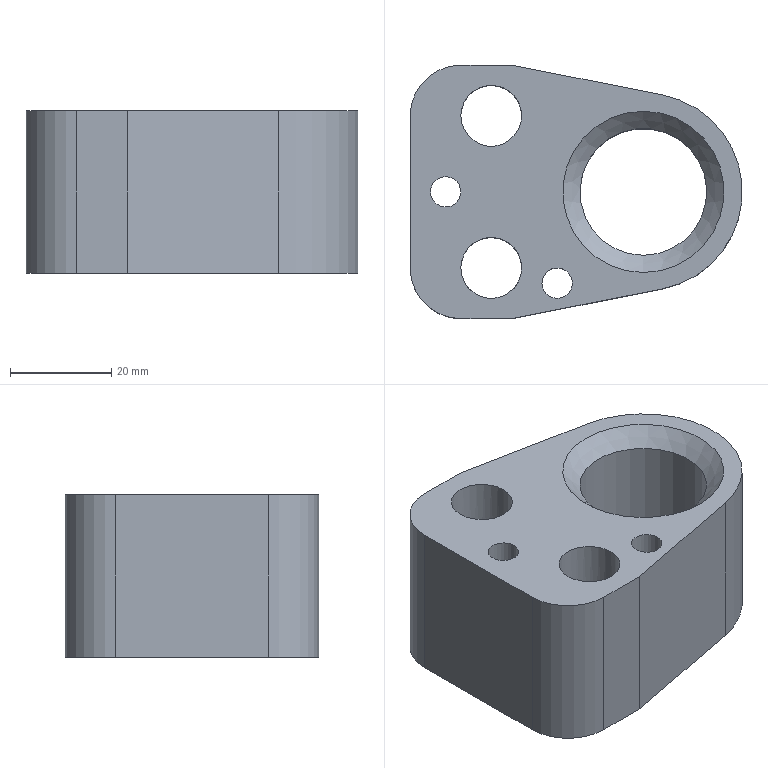Part | NX | features solid 2 | 1 solid | 24 faces | box 65.5 x 50 x 32 mm | volume 58243 mm3 | cylinder 12 | plane 11 | cone 1 | commonest cylinder face diameters 6 x2 8 x2 12 x2 17 x2 20 x2 25 x1
STEP:
#1=CARTESIAN_POINT('',(-607.367,572.653,75.));
#2=VERTEX_POINT('',#1);
#3=CARTESIAN_POINT('',(-607.367,576.653,75.));
#4=DIRECTION('',(0.,0.,-1.));
#5=DIRECTION('',(0.,-1.,0.));
#6=AXIS2_PLACEMENT_3D('',#3,#4,#5);
#7=CIRCLE('',#6,4.);
#8=EDGE_CURVE('',#2,#2,#7,.F.);
#9=ORIENTED_EDGE('',*,*,#8,.T.);
#10=EDGE_LOOP('',(#9));
#11=FACE_BOUND('',#10,.T.);
#12=CARTESIAN_POINT('',(-606.867,591.653,75.));
#13=VERTEX_POINT('',#12);
#14=CARTESIAN_POINT('',(-598.367,591.653,75.));
#15=DIRECTION('',(0.,0.,1.));
#16=DIRECTION('',(-1.,0.,0.));
#17=AXIS2_PLACEMENT_3D('',#14,#15,#16);
#18=CIRCLE('',#17,8.5);
#19=EDGE_CURVE('',#13,#13,#18,.T.);
#20=ORIENTED_EDGE('',*,*,#19,.T.);
#21=EDGE_LOOP('',(#20));
#22=FACE_BOUND('',#21,.T.);
#23=CARTESIAN_POINT('',(-606.867,561.653,75.));
#24=VERTEX_POINT('',#23);
#25=CARTESIAN_POINT('',(-598.367,561.653,75.));
#26=DIRECTION('',(0.,0.,1.));
#27=DIRECTION('',(-1.,0.,0.));
#28=AXIS2_PLACEMENT_3D('',#25,#26,#27);
#29=CIRCLE('',#28,8.5);
#30=EDGE_CURVE('',#24,#24,#29,.T.);
#31=ORIENTED_EDGE('',*,*,#30,.T.);
#32=EDGE_LOOP('',(#31));
#33=FACE_BOUND('',#32,.T.);
#34=CARTESIAN_POINT('',(-568.367,564.153,75.));
#35=VERTEX_POINT('',#34);
#36=CARTESIAN_POINT('',(-568.367,576.653,75.));
#37=DIRECTION('',(0.,0.,-1.));
#38=DIRECTION('',(0.,-1.,0.));
#39=AXIS2_PLACEMENT_3D('',#36,#37,#38);
#40=CIRCLE('',#39,12.5);
#41=EDGE_CURVE('',#35,#35,#40,.T.);
#42=ORIENTED_EDGE('',*,*,#41,.F.);
#43=EDGE_LOOP('',(#42));
#44=FACE_BOUND('',#43,.T.);
#45=CARTESIAN_POINT('',(-604.367,601.653,75.));
#46=VERTEX_POINT('',#45);
#47=CARTESIAN_POINT('',(-614.367,591.653,75.));
#48=VERTEX_POINT('',#47);
#49=CARTESIAN_POINT('',(-604.367,591.653,75.));
#50=DIRECTION('',(0.,0.,1.));
#51=DIRECTION('',(-1.,0.,0.));
#52=AXIS2_PLACEMENT_3D('',#49,#50,#51);
#53=CIRCLE('',#52,10.);
#54=EDGE_CURVE('',#46,#48,#53,.T.);
#55=ORIENTED_EDGE('',*,*,#54,.F.);
#56=CARTESIAN_POINT('',(-594.367,601.653,75.));
#57=VERTEX_POINT('',#56);
#58=CARTESIAN_POINT('',(-594.367,601.653,75.));
#59=DIRECTION('',(-1.,0.,0.));
#60=VECTOR('',#59,1000.);
#61=LINE('',#58,#60);
#62=EDGE_CURVE('',#57,#46,#61,.T.);
#63=ORIENTED_EDGE('',*,*,#62,.F.);
#64=CARTESIAN_POINT('',(-564.595,595.785,75.));
#65=VERTEX_POINT('',#64);
#66=CARTESIAN_POINT('',(-564.595,595.785,75.));
#67=DIRECTION('',(-0.9811,0.1934,0.));
#68=VECTOR('',#67,1000.);
#69=LINE('',#66,#68);
#70=EDGE_CURVE('',#65,#57,#69,.T.);
#71=ORIENTED_EDGE('',*,*,#70,.F.);
#72=CARTESIAN_POINT('',(-564.595,557.521,75.));
#73=VERTEX_POINT('',#72);
#74=CARTESIAN_POINT('',(-568.367,576.653,75.));
#75=DIRECTION('',(0.,0.,1.));
#76=DIRECTION('',(-1.,0.,0.));
#77=AXIS2_PLACEMENT_3D('',#74,#75,#76);
#78=CIRCLE('',#77,19.5);
#79=EDGE_CURVE('',#73,#65,#78,.T.);
#80=ORIENTED_EDGE('',*,*,#79,.F.);
#81=CARTESIAN_POINT('',(-594.367,551.653,75.));
#82=VERTEX_POINT('',#81);
#83=CARTESIAN_POINT('',(-564.595,557.521,75.));
#84=DIRECTION('',(-0.9811,-0.1934,0.));
#85=VECTOR('',#84,1000.);
#86=LINE('',#83,#85);
#87=EDGE_CURVE('',#73,#82,#86,.T.);
#88=ORIENTED_EDGE('',*,*,#87,.T.);
#89=CARTESIAN_POINT('',(-604.367,551.653,75.));
#90=VERTEX_POINT('',#89);
#91=CARTESIAN_POINT('',(-594.367,551.653,75.));
#92=DIRECTION('',(-1.,0.,0.));
#93=VECTOR('',#92,1000.);
#94=LINE('',#91,#93);
#95=EDGE_CURVE('',#82,#90,#94,.T.);
#96=ORIENTED_EDGE('',*,*,#95,.T.);
#97=CARTESIAN_POINT('',(-614.367,561.653,75.));
#98=VERTEX_POINT('',#97);
#99=CARTESIAN_POINT('',(-604.367,561.653,75.));
#100=DIRECTION('',(0.,0.,1.));
#101=DIRECTION('',(-1.,0.,0.));
#102=AXIS2_PLACEMENT_3D('',#99,#100,#101);
#103=CIRCLE('',#102,10.);
#104=EDGE_CURVE('',#98,#90,#103,.T.);
#105=ORIENTED_EDGE('',*,*,#104,.F.);
#106=CARTESIAN_POINT('',(-614.367,561.653,75.));
#107=DIRECTION('',(0.,1.,0.));
#108=VECTOR('',#107,1000.);
#109=LINE('',#106,#108);
#110=EDGE_CURVE('',#98,#48,#109,.T.);
#111=ORIENTED_EDGE('',*,*,#110,.T.);
#112=EDGE_LOOP('',(#55,#63,#71,#80,#88,#96,#105,#111));
#113=FACE_BOUND('',#112,.T.);
#114=CARTESIAN_POINT('',(-585.367,554.653,75.));
#115=VERTEX_POINT('',#114);
#116=CARTESIAN_POINT('',(-585.367,558.653,75.));
#117=DIRECTION('',(0.,0.,-1.));
#118=DIRECTION('',(0.,-1.,0.));
#119=AXIS2_PLACEMENT_3D('',#116,#117,#118);
#120=CIRCLE('',#119,4.);
#121=EDGE_CURVE('',#115,#115,#120,.F.);
#122=ORIENTED_EDGE('',*,*,#121,.T.);
#123=EDGE_LOOP('',(#122));
#124=FACE_BOUND('',#123,.T.);
#125=CARTESIAN_POINT('',(-604.367,591.653,75.));
#126=DIRECTION('',(0.,0.,-1.));
#127=DIRECTION('',(0.,1.,0.));
#128=AXIS2_PLACEMENT_3D('',#125,#126,#127);
#129=PLANE('',#128);
#130=ADVANCED_FACE('',(#11,#22,#33,#44,#113,#124),#129,.T.);
#131=CARTESIAN_POINT('',(-604.367,591.653,107.));
#132=VERTEX_POINT('',#131);
#133=CARTESIAN_POINT('',(-598.367,591.653,107.));
#134=DIRECTION('',(0.,0.,1.));
#135=DIRECTION('',(-1.,0.,0.));
#136=AXIS2_PLACEMENT_3D('',#133,#134,#135);
#137=CIRCLE('',#136,6.);
#138=EDGE_CURVE('',#132,#132,#137,.T.);
#139=ORIENTED_EDGE('',*,*,#138,.T.);
#140=EDGE_LOOP('',(#139));
#141=FACE_BOUND('',#140,.T.);
#142=CARTESIAN_POINT('',(-598.367,597.653,87.));
#143=VERTEX_POINT('',#142);
#144=CARTESIAN_POINT('',(-598.367,591.653,87.));
#145=DIRECTION('',(0.,0.,1.));
#146=DIRECTION('',(0.,1.,0.));
#147=AXIS2_PLACEMENT_3D('',#144,#145,#146);
#148=CIRCLE('',#147,6.);
#149=EDGE_CURVE('',#143,#143,#148,.T.);
#150=ORIENTED_EDGE('',*,*,#149,.F.);
#151=EDGE_LOOP('',(#150));
#152=FACE_BOUND('',#151,.T.);
#153=CARTESIAN_POINT('',(-598.367,591.653,75.));
#154=DIRECTION('',(0.,0.,1.));
#155=DIRECTION('',(0.,-1.,0.));
#156=AXIS2_PLACEMENT_3D('',#153,#154,#155);
#157=CYLINDRICAL_SURFACE('',#156,6.);
#158=ADVANCED_FACE('',(#141,#152),#157,.F.);
#159=CARTESIAN_POINT('',(-604.367,561.653,107.));
#160=VERTEX_POINT('',#159);
#161=CARTESIAN_POINT('',(-598.367,561.653,107.));
#162=DIRECTION('',(0.,0.,1.));
#163=DIRECTION('',(-1.,0.,0.));
#164=AXIS2_PLACEMENT_3D('',#161,#162,#163);
#165=CIRCLE('',#164,6.);
#166=EDGE_CURVE('',#160,#160,#165,.T.);
#167=ORIENTED_EDGE('',*,*,#166,.T.);
#168=EDGE_LOOP('',(#167));
#169=FACE_BOUND('',#168,.T.);
#170=CARTESIAN_POINT('',(-598.367,567.653,87.));
#171=VERTEX_POINT('',#170);
#172=CARTESIAN_POINT('',(-598.367,561.653,87.));
#173=DIRECTION('',(0.,0.,1.));
#174=DIRECTION('',(0.,1.,0.));
#175=AXIS2_PLACEMENT_3D('',#172,#173,#174);
#176=CIRCLE('',#175,6.);
#177=EDGE_CURVE('',#171,#171,#176,.T.);
#178=ORIENTED_EDGE('',*,*,#177,.F.);
#179=EDGE_LOOP('',(#178));
#180=FACE_BOUND('',#179,.T.);
#181=CARTESIAN_POINT('',(-598.367,561.653,75.));
#182=DIRECTION('',(0.,0.,1.));
#183=DIRECTION('',(0.,-1.,0.));
#184=AXIS2_PLACEMENT_3D('',#181,#182,#183);
#185=CYLINDRICAL_SURFACE('',#184,6.);
#186=ADVANCED_FACE('',(#169,#180),#185,.F.);
#187=CARTESIAN_POINT('',(-588.367,558.653,107.));
#188=VERTEX_POINT('',#187);
#189=CARTESIAN_POINT('',(-585.367,558.653,107.));
#190=DIRECTION('',(0.,0.,1.));
#191=DIRECTION('',(-1.,0.,0.));
#192=AXIS2_PLACEMENT_3D('',#189,#190,#191);
#193=CIRCLE('',#192,3.);
#194=EDGE_CURVE('',#188,#188,#193,.T.);
#195=ORIENTED_EDGE('',*,*,#194,.F.);
#196=EDGE_LOOP('',(#195));
#197=FACE_BOUND('',#196,.T.);
#198=ORIENTED_EDGE('',*,*,#166,.F.);
#199=EDGE_LOOP('',(#198));
#200=FACE_BOUND('',#199,.T.);
#201=CARTESIAN_POINT('',(-568.367,592.553,107.));
#202=VERTEX_POINT('',#201);
#203=CARTESIAN_POINT('',(-568.367,576.653,107.));
#204=DIRECTION('',(0.,0.,1.));
#205=DIRECTION('',(0.,1.,0.));
#206=AXIS2_PLACEMENT_3D('',#203,#204,#205);
#207=CIRCLE('',#206,15.9);
#208=EDGE_CURVE('',#202,#202,#207,.T.);
#209=ORIENTED_EDGE('',*,*,#208,.F.);
#210=EDGE_LOOP('',(#209));
#211=FACE_BOUND('',#210,.T.);
#212=CARTESIAN_POINT('',(-604.367,601.653,107.));
#213=VERTEX_POINT('',#212);
#214=CARTESIAN_POINT('',(-614.367,591.653,107.));
#215=VERTEX_POINT('',#214);
#216=CARTESIAN_POINT('',(-604.367,591.653,107.));
#217=DIRECTION('',(0.,0.,1.));
#218=DIRECTION('',(-1.,0.,0.));
#219=AXIS2_PLACEMENT_3D('',#216,#217,#218);
#220=CIRCLE('',#219,10.);
#221=EDGE_CURVE('',#213,#215,#220,.T.);
#222=ORIENTED_EDGE('',*,*,#221,.T.);
#223=CARTESIAN_POINT('',(-614.367,561.653,107.));
#224=VERTEX_POINT('',#223);
#225=CARTESIAN_POINT('',(-614.367,561.653,107.));
#226=DIRECTION('',(0.,1.,0.));
#227=VECTOR('',#226,1000.);
#228=LINE('',#225,#227);
#229=EDGE_CURVE('',#224,#215,#228,.T.);
#230=ORIENTED_EDGE('',*,*,#229,.F.);
#231=CARTESIAN_POINT('',(-604.367,551.653,107.));
#232=VERTEX_POINT('',#231);
#233=CARTESIAN_POINT('',(-604.367,561.653,107.));
#234=DIRECTION('',(0.,0.,1.));
#235=DIRECTION('',(-1.,0.,0.));
#236=AXIS2_PLACEMENT_3D('',#233,#234,#235);
#237=CIRCLE('',#236,10.);
#238=EDGE_CURVE('',#224,#232,#237,.T.);
#239=ORIENTED_EDGE('',*,*,#238,.T.);
#240=CARTESIAN_POINT('',(-594.367,551.653,107.));
#241=VERTEX_POINT('',#240);
#242=CARTESIAN_POINT('',(-594.367,551.653,107.));
#243=DIRECTION('',(-1.,0.,0.));
#244=VECTOR('',#243,1000.);
#245=LINE('',#242,#244);
#246=EDGE_CURVE('',#241,#232,#245,.T.);
#247=ORIENTED_EDGE('',*,*,#246,.F.);
#248=CARTESIAN_POINT('',(-564.595,557.521,107.));
#249=VERTEX_POINT('',#248);
#250=CARTESIAN_POINT('',(-564.595,557.521,107.));
#251=DIRECTION('',(-0.9811,-0.1934,0.));
#252=VECTOR('',#251,1000.);
#253=LINE('',#250,#252);
#254=EDGE_CURVE('',#249,#241,#253,.T.);
#255=ORIENTED_EDGE('',*,*,#254,.F.);
#256=CARTESIAN_POINT('',(-564.595,595.785,107.));
#257=VERTEX_POINT('',#256);
#258=CARTESIAN_POINT('',(-568.367,576.653,107.));
#259=DIRECTION('',(0.,0.,1.));
#260=DIRECTION('',(-1.,0.,0.));
#261=AXIS2_PLACEMENT_3D('',#258,#259,#260);
#262=CIRCLE('',#261,19.5);
#263=EDGE_CURVE('',#249,#257,#262,.T.);
#264=ORIENTED_EDGE('',*,*,#263,.T.);
#265=CARTESIAN_POINT('',(-594.367,601.653,107.));
#266=VERTEX_POINT('',#265);
#267=CARTESIAN_POINT('',(-564.595,595.785,107.));
#268=DIRECTION('',(-0.9811,0.1934,0.));
#269=VECTOR('',#268,1000.);
#270=LINE('',#267,#269);
#271=EDGE_CURVE('',#257,#266,#270,.T.);
#272=ORIENTED_EDGE('',*,*,#271,.T.);
#273=CARTESIAN_POINT('',(-594.367,601.653,107.));
#274=DIRECTION('',(-1.,0.,0.));
#275=VECTOR('',#274,1000.);
#276=LINE('',#273,#275);
#277=EDGE_CURVE('',#266,#213,#276,.T.);
#278=ORIENTED_EDGE('',*,*,#277,.T.);
#279=EDGE_LOOP('',(#222,#230,#239,#247,#255,#264,#272,#278));
#280=FACE_BOUND('',#279,.T.);
#281=ORIENTED_EDGE('',*,*,#138,.F.);
#282=EDGE_LOOP('',(#281));
#283=FACE_BOUND('',#282,.T.);
#284=CARTESIAN_POINT('',(-610.367,576.653,107.));
#285=VERTEX_POINT('',#284);
#286=CARTESIAN_POINT('',(-607.367,576.653,107.));
#287=DIRECTION('',(0.,0.,1.));
#288=DIRECTION('',(-1.,0.,0.));
#289=AXIS2_PLACEMENT_3D('',#286,#287,#288);
#290=CIRCLE('',#289,3.);
#291=EDGE_CURVE('',#285,#285,#290,.T.);
#292=ORIENTED_EDGE('',*,*,#291,.F.);
#293=EDGE_LOOP('',(#292));
#294=FACE_BOUND('',#293,.T.);
#295=CARTESIAN_POINT('',(-604.367,591.653,107.));
#296=DIRECTION('',(0.,0.,-1.));
#297=DIRECTION('',(0.,1.,0.));
#298=AXIS2_PLACEMENT_3D('',#295,#296,#297);
#299=PLANE('',#298);
#300=ADVANCED_FACE('',(#197,#200,#211,#280,#283,#294),#299,.F.);
#301=ORIENTED_EDGE('',*,*,#221,.F.);
#302=CARTESIAN_POINT('',(-604.367,601.653,75.));
#303=DIRECTION('',(0.,0.,1.));
#304=VECTOR('',#303,1000.);
#305=LINE('',#302,#304);
#306=EDGE_CURVE('',#46,#213,#305,.T.);
#307=ORIENTED_EDGE('',*,*,#306,.F.);
#308=ORIENTED_EDGE('',*,*,#54,.T.);
#309=CARTESIAN_POINT('',(-614.367,591.653,75.));
#310=DIRECTION('',(0.,0.,1.));
#311=VECTOR('',#310,1000.);
#312=LINE('',#309,#311);
#313=EDGE_CURVE('',#48,#215,#312,.T.);
#314=ORIENTED_EDGE('',*,*,#313,.T.);
#315=EDGE_LOOP('',(#301,#307,#308,#314));
#316=FACE_BOUND('',#315,.T.);
#317=CARTESIAN_POINT('',(-604.367,591.653,75.));
#318=DIRECTION('',(0.,0.,1.));
#319=DIRECTION('',(0.,-1.,0.));
#320=AXIS2_PLACEMENT_3D('',#317,#318,#319);
#321=CYLINDRICAL_SURFACE('',#320,10.);
#322=ADVANCED_FACE('',(#316),#321,.T.);
#323=ORIENTED_EDGE('',*,*,#229,.T.);
#324=ORIENTED_EDGE('',*,*,#313,.F.);
#325=ORIENTED_EDGE('',*,*,#110,.F.);
#326=CARTESIAN_POINT('',(-614.367,561.653,75.));
#327=DIRECTION('',(0.,0.,1.));
#328=VECTOR('',#327,1000.);
#329=LINE('',#326,#328);
#330=EDGE_CURVE('',#98,#224,#329,.T.);
#331=ORIENTED_EDGE('',*,*,#330,.T.);
#332=EDGE_LOOP('',(#323,#324,#325,#331));
#333=FACE_BOUND('',#332,.T.);
#334=CARTESIAN_POINT('',(-614.367,561.653,75.));
#335=DIRECTION('',(-1.,0.,0.));
#336=DIRECTION('',(0.,0.,1.));
#337=AXIS2_PLACEMENT_3D('',#334,#335,#336);
#338=PLANE('',#337);
#339=ADVANCED_FACE('',(#333),#338,.T.);
#340=ORIENTED_EDGE('',*,*,#238,.F.);
#341=ORIENTED_EDGE('',*,*,#330,.F.);
#342=ORIENTED_EDGE('',*,*,#104,.T.);
#343=CARTESIAN_POINT('',(-604.367,551.653,75.));
#344=DIRECTION('',(0.,0.,1.));
#345=VECTOR('',#344,1000.);
#346=LINE('',#343,#345);
#347=EDGE_CURVE('',#90,#232,#346,.T.);
#348=ORIENTED_EDGE('',*,*,#347,.T.);
#349=EDGE_LOOP('',(#340,#341,#342,#348));
#350=FACE_BOUND('',#349,.T.);
#351=CARTESIAN_POINT('',(-604.367,561.653,75.));
#352=DIRECTION('',(0.,0.,1.));
#353=DIRECTION('',(0.,-1.,0.));
#354=AXIS2_PLACEMENT_3D('',#351,#352,#353);
#355=CYLINDRICAL_SURFACE('',#354,10.);
#356=ADVANCED_FACE('',(#350),#355,.T.);
#357=ORIENTED_EDGE('',*,*,#246,.T.);
#358=ORIENTED_EDGE('',*,*,#347,.F.);
#359=ORIENTED_EDGE('',*,*,#95,.F.);
#360=CARTESIAN_POINT('',(-594.367,551.653,75.));
#361=DIRECTION('',(0.,0.,1.));
#362=VECTOR('',#361,1000.);
#363=LINE('',#360,#362);
#364=EDGE_CURVE('',#82,#241,#363,.T.);
#365=ORIENTED_EDGE('',*,*,#364,.T.);
#366=EDGE_LOOP('',(#357,#358,#359,#365));
#367=FACE_BOUND('',#366,.T.);
#368=CARTESIAN_POINT('',(-594.367,551.653,75.));
#369=DIRECTION('',(0.,-1.,0.));
#370=DIRECTION('',(0.,0.,-1.));
#371=AXIS2_PLACEMENT_3D('',#368,#369,#370);
#372=PLANE('',#371);
#373=ADVANCED_FACE('',(#367),#372,.T.);
#374=ORIENTED_EDGE('',*,*,#254,.T.);
#375=ORIENTED_EDGE('',*,*,#364,.F.);
#376=ORIENTED_EDGE('',*,*,#87,.F.);
#377=CARTESIAN_POINT('',(-564.595,557.521,75.));
#378=DIRECTION('',(0.,0.,1.));
#379=VECTOR('',#378,1000.);
#380=LINE('',#377,#379);
#381=EDGE_CURVE('',#73,#249,#380,.T.);
#382=ORIENTED_EDGE('',*,*,#381,.T.);
#383=EDGE_LOOP('',(#374,#375,#376,#382));
#384=FACE_BOUND('',#383,.T.);
#385=CARTESIAN_POINT('',(-564.595,557.521,75.));
#386=DIRECTION('',(0.1934,-0.9811,0.));
#387=DIRECTION('',(-0.9811,-0.1934,0.));
#388=AXIS2_PLACEMENT_3D('',#385,#386,#387);
#389=PLANE('',#388);
#390=ADVANCED_FACE('',(#384),#389,.T.);
#391=ORIENTED_EDGE('',*,*,#263,.F.);
#392=ORIENTED_EDGE('',*,*,#381,.F.);
#393=ORIENTED_EDGE('',*,*,#79,.T.);
#394=CARTESIAN_POINT('',(-564.595,595.785,75.));
#395=DIRECTION('',(0.,0.,1.));
#396=VECTOR('',#395,1000.);
#397=LINE('',#394,#396);
#398=EDGE_CURVE('',#65,#257,#397,.T.);
#399=ORIENTED_EDGE('',*,*,#398,.T.);
#400=EDGE_LOOP('',(#391,#392,#393,#399));
#401=FACE_BOUND('',#400,.T.);
#402=CARTESIAN_POINT('',(-568.367,576.653,75.));
#403=DIRECTION('',(0.,0.,1.));
#404=DIRECTION('',(0.,-1.,0.));
#405=AXIS2_PLACEMENT_3D('',#402,#403,#404);
#406=CYLINDRICAL_SURFACE('',#405,19.5);
#407=ADVANCED_FACE('',(#401),#406,.T.);
#408=ORIENTED_EDGE('',*,*,#271,.F.);
#409=ORIENTED_EDGE('',*,*,#398,.F.);
#410=ORIENTED_EDGE('',*,*,#70,.T.);
#411=CARTESIAN_POINT('',(-594.367,601.653,75.));
#412=DIRECTION('',(0.,0.,1.));
#413=VECTOR('',#412,1000.);
#414=LINE('',#411,#413);
#415=EDGE_CURVE('',#57,#266,#414,.T.);
#416=ORIENTED_EDGE('',*,*,#415,.T.);
#417=EDGE_LOOP('',(#408,#409,#410,#416));
#418=FACE_BOUND('',#417,.T.);
#419=CARTESIAN_POINT('',(-564.595,595.785,75.));
#420=DIRECTION('',(-0.1934,-0.9811,0.));
#421=DIRECTION('',(-0.9811,0.1934,0.));
#422=AXIS2_PLACEMENT_3D('',#419,#420,#421);
#423=PLANE('',#422);
#424=ADVANCED_FACE('',(#418),#423,.F.);
#425=ORIENTED_EDGE('',*,*,#277,.F.);
#426=ORIENTED_EDGE('',*,*,#415,.F.);
#427=ORIENTED_EDGE('',*,*,#62,.T.);
#428=ORIENTED_EDGE('',*,*,#306,.T.);
#429=EDGE_LOOP('',(#425,#426,#427,#428));
#430=FACE_BOUND('',#429,.T.);
#431=CARTESIAN_POINT('',(-594.367,601.653,75.));
#432=DIRECTION('',(0.,-1.,0.));
#433=DIRECTION('',(-1.,0.,0.));
#434=AXIS2_PLACEMENT_3D('',#431,#432,#433);
#435=PLANE('',#434);
#436=ADVANCED_FACE('',(#430),#435,.F.);
#437=ORIENTED_EDGE('',*,*,#41,.T.);
#438=EDGE_LOOP('',(#437));
#439=FACE_BOUND('',#438,.T.);
#440=CARTESIAN_POINT('',(-568.367,564.153,103.6));
#441=VERTEX_POINT('',#440);
#442=CARTESIAN_POINT('',(-568.367,576.653,103.6));
#443=DIRECTION('',(0.,0.,1.));
#444=DIRECTION('',(0.,-1.,0.));
#445=AXIS2_PLACEMENT_3D('',#442,#443,#444);
#446=CIRCLE('',#445,12.5);
#447=EDGE_CURVE('',#441,#441,#446,.T.);
#448=ORIENTED_EDGE('',*,*,#447,.T.);
#449=EDGE_LOOP('',(#448));
#450=FACE_BOUND('',#449,.T.);
#451=CARTESIAN_POINT('',(-568.367,576.653,75.));
#452=DIRECTION('',(0.,0.,1.));
#453=DIRECTION('',(0.,-1.,0.));
#454=AXIS2_PLACEMENT_3D('',#451,#452,#453);
#455=CYLINDRICAL_SURFACE('',#454,12.5);
#456=ADVANCED_FACE('',(#439,#450),#455,.F.);
#457=ORIENTED_EDGE('',*,*,#208,.T.);
#458=EDGE_LOOP('',(#457));
#459=FACE_BOUND('',#458,.T.);
#460=ORIENTED_EDGE('',*,*,#447,.F.);
#461=EDGE_LOOP('',(#460));
#462=FACE_BOUND('',#461,.T.);
#463=CARTESIAN_POINT('',(-568.367,576.653,103.6));
#464=DIRECTION('',(0.,0.,1.));
#465=DIRECTION('',(0.,-1.,0.));
#466=AXIS2_PLACEMENT_3D('',#463,#464,#465);
#467=CONICAL_SURFACE('',#466,12.5,0.7854);
#468=ADVANCED_FACE('',(#459,#462),#467,.F.);
#469=CARTESIAN_POINT('',(-588.367,558.653,95.));
#470=VERTEX_POINT('',#469);
#471=CARTESIAN_POINT('',(-585.367,558.653,95.));
#472=DIRECTION('',(0.,0.,1.));
#473=DIRECTION('',(-1.,0.,0.));
#474=AXIS2_PLACEMENT_3D('',#471,#472,#473);
#475=CIRCLE('',#474,3.);
#476=EDGE_CURVE('',#470,#470,#475,.T.);
#477=ORIENTED_EDGE('',*,*,#476,.F.);
#478=EDGE_LOOP('',(#477));
#479=FACE_BOUND('',#478,.T.);
#480=ORIENTED_EDGE('',*,*,#194,.T.);
#481=EDGE_LOOP('',(#480));
#482=FACE_BOUND('',#481,.T.);
#483=CARTESIAN_POINT('',(-585.367,558.653,75.));
#484=DIRECTION('',(0.,0.,1.));
#485=DIRECTION('',(0.,-1.,0.));
#486=AXIS2_PLACEMENT_3D('',#483,#484,#485);
#487=CYLINDRICAL_SURFACE('',#486,3.);
#488=ADVANCED_FACE('',(#479,#482),#487,.F.);
#489=CARTESIAN_POINT('',(-610.367,576.653,95.));
#490=VERTEX_POINT('',#489);
#491=CARTESIAN_POINT('',(-607.367,576.653,95.));
#492=DIRECTION('',(0.,0.,1.));
#493=DIRECTION('',(-1.,0.,0.));
#494=AXIS2_PLACEMENT_3D('',#491,#492,#493);
#495=CIRCLE('',#494,3.);
#496=EDGE_CURVE('',#490,#490,#495,.T.);
#497=ORIENTED_EDGE('',*,*,#496,.F.);
#498=EDGE_LOOP('',(#497));
#499=FACE_BOUND('',#498,.T.);
#500=ORIENTED_EDGE('',*,*,#291,.T.);
#501=EDGE_LOOP('',(#500));
#502=FACE_BOUND('',#501,.T.);
#503=CARTESIAN_POINT('',(-607.367,576.653,75.));
#504=DIRECTION('',(0.,0.,1.));
#505=DIRECTION('',(0.,-1.,0.));
#506=AXIS2_PLACEMENT_3D('',#503,#504,#505);
#507=CYLINDRICAL_SURFACE('',#506,3.);
#508=ADVANCED_FACE('',(#499,#502),#507,.F.);
#509=CARTESIAN_POINT('',(-606.867,561.653,87.));
#510=VERTEX_POINT('',#509);
#511=CARTESIAN_POINT('',(-598.367,561.653,87.));
#512=DIRECTION('',(0.,0.,1.));
#513=DIRECTION('',(-1.,0.,0.));
#514=AXIS2_PLACEMENT_3D('',#511,#512,#513);
#515=CIRCLE('',#514,8.5);
#516=EDGE_CURVE('',#510,#510,#515,.T.);
#517=ORIENTED_EDGE('',*,*,#516,.T.);
#518=EDGE_LOOP('',(#517));
#519=FACE_BOUND('',#518,.T.);
#520=ORIENTED_EDGE('',*,*,#30,.F.);
#521=EDGE_LOOP('',(#520));
#522=FACE_BOUND('',#521,.T.);
#523=CARTESIAN_POINT('',(-598.367,561.653,87.));
#524=DIRECTION('',(0.,0.,-1.));
#525=DIRECTION('',(0.,1.,0.));
#526=AXIS2_PLACEMENT_3D('',#523,#524,#525);
#527=CYLINDRICAL_SURFACE('',#526,8.5);
#528=ADVANCED_FACE('',(#519,#522),#527,.F.);
#529=ORIENTED_EDGE('',*,*,#177,.T.);
#530=EDGE_LOOP('',(#529));
#531=FACE_BOUND('',#530,.T.);
#532=ORIENTED_EDGE('',*,*,#516,.F.);
#533=EDGE_LOOP('',(#532));
#534=FACE_BOUND('',#533,.T.);
#535=CARTESIAN_POINT('',(-598.367,561.653,87.));
#536=DIRECTION('',(0.,0.,-1.));
#537=DIRECTION('',(0.,1.,0.));
#538=AXIS2_PLACEMENT_3D('',#535,#536,#537);
#539=PLANE('',#538);
#540=ADVANCED_FACE('',(#531,#534),#539,.T.);
#541=CARTESIAN_POINT('',(-606.867,591.653,87.));
#542=VERTEX_POINT('',#541);
#543=CARTESIAN_POINT('',(-598.367,591.653,87.));
#544=DIRECTION('',(0.,0.,1.));
#545=DIRECTION('',(-1.,0.,0.));
#546=AXIS2_PLACEMENT_3D('',#543,#544,#545);
#547=CIRCLE('',#546,8.5);
#548=EDGE_CURVE('',#542,#542,#547,.T.);
#549=ORIENTED_EDGE('',*,*,#548,.T.);
#550=EDGE_LOOP('',(#549));
#551=FACE_BOUND('',#550,.T.);
#552=ORIENTED_EDGE('',*,*,#19,.F.);
#553=EDGE_LOOP('',(#552));
#554=FACE_BOUND('',#553,.T.);
#555=CARTESIAN_POINT('',(-598.367,591.653,87.));
#556=DIRECTION('',(0.,0.,-1.));
#557=DIRECTION('',(0.,1.,0.));
#558=AXIS2_PLACEMENT_3D('',#555,#556,#557);
#559=CYLINDRICAL_SURFACE('',#558,8.5);
#560=ADVANCED_FACE('',(#551,#554),#559,.F.);
#561=ORIENTED_EDGE('',*,*,#149,.T.);
#562=EDGE_LOOP('',(#561));
#563=FACE_BOUND('',#562,.T.);
#564=ORIENTED_EDGE('',*,*,#548,.F.);
#565=EDGE_LOOP('',(#564));
#566=FACE_BOUND('',#565,.T.);
#567=CARTESIAN_POINT('',(-598.367,591.653,87.));
#568=DIRECTION('',(0.,0.,-1.));
#569=DIRECTION('',(0.,1.,0.));
#570=AXIS2_PLACEMENT_3D('',#567,#568,#569);
#571=PLANE('',#570);
#572=ADVANCED_FACE('',(#563,#566),#571,.T.);
#573=CARTESIAN_POINT('',(-607.367,572.653,95.));
#574=VERTEX_POINT('',#573);
#575=CARTESIAN_POINT('',(-607.367,576.653,95.));
#576=DIRECTION('',(0.,0.,-1.));
#577=DIRECTION('',(0.,-1.,0.));
#578=AXIS2_PLACEMENT_3D('',#575,#576,#577);
#579=CIRCLE('',#578,4.);
#580=EDGE_CURVE('',#574,#574,#579,.F.);
#581=ORIENTED_EDGE('',*,*,#580,.F.);
#582=EDGE_LOOP('',(#581));
#583=FACE_BOUND('',#582,.T.);
#584=ORIENTED_EDGE('',*,*,#496,.T.);
#585=EDGE_LOOP('',(#584));
#586=FACE_BOUND('',#585,.T.);
#587=CARTESIAN_POINT('',(-607.367,576.653,95.));
#588=DIRECTION('',(0.,0.,1.));
#589=DIRECTION('',(0.,-1.,0.));
#590=AXIS2_PLACEMENT_3D('',#587,#588,#589);
#591=PLANE('',#590);
#592=ADVANCED_FACE('',(#583,#586),#591,.F.);
#593=ORIENTED_EDGE('',*,*,#580,.T.);
#594=EDGE_LOOP('',(#593));
#595=FACE_BOUND('',#594,.T.);
#596=ORIENTED_EDGE('',*,*,#8,.F.);
#597=EDGE_LOOP('',(#596));
#598=FACE_BOUND('',#597,.T.);
#599=CARTESIAN_POINT('',(-607.367,576.653,75.));
#600=DIRECTION('',(0.,0.,1.));
#601=DIRECTION('',(0.,-1.,0.));
#602=AXIS2_PLACEMENT_3D('',#599,#600,#601);
#603=CYLINDRICAL_SURFACE('',#602,4.);
#604=ADVANCED_FACE('',(#595,#598),#603,.F.);
#605=CARTESIAN_POINT('',(-585.367,554.653,95.));
#606=VERTEX_POINT('',#605);
#607=CARTESIAN_POINT('',(-585.367,558.653,95.));
#608=DIRECTION('',(0.,0.,-1.));
#609=DIRECTION('',(0.,-1.,0.));
#610=AXIS2_PLACEMENT_3D('',#607,#608,#609);
#611=CIRCLE('',#610,4.);
#612=EDGE_CURVE('',#606,#606,#611,.F.);
#613=ORIENTED_EDGE('',*,*,#612,.F.);
#614=EDGE_LOOP('',(#613));
#615=FACE_BOUND('',#614,.T.);
#616=ORIENTED_EDGE('',*,*,#476,.T.);
#617=EDGE_LOOP('',(#616));
#618=FACE_BOUND('',#617,.T.);
#619=CARTESIAN_POINT('',(-585.367,558.653,95.));
#620=DIRECTION('',(0.,0.,1.));
#621=DIRECTION('',(0.,-1.,0.));
#622=AXIS2_PLACEMENT_3D('',#619,#620,#621);
#623=PLANE('',#622);
#624=ADVANCED_FACE('',(#615,#618),#623,.F.);
#625=ORIENTED_EDGE('',*,*,#612,.T.);
#626=EDGE_LOOP('',(#625));
#627=FACE_BOUND('',#626,.T.);
#628=ORIENTED_EDGE('',*,*,#121,.F.);
#629=EDGE_LOOP('',(#628));
#630=FACE_BOUND('',#629,.T.);
#631=CARTESIAN_POINT('',(-585.367,558.653,75.));
#632=DIRECTION('',(0.,0.,1.));
#633=DIRECTION('',(0.,-1.,0.));
#634=AXIS2_PLACEMENT_3D('',#631,#632,#633);
#635=CYLINDRICAL_SURFACE('',#634,4.);
#636=ADVANCED_FACE('',(#627,#630),#635,.F.);
#637=CLOSED_SHELL('',(#130,#158,#186,#300,#322,#339,#356,#373,#390,#407,#424,#436,#456,#468,#488,#508,#528,#540,#560,#572,#592,#604,#624,#636));
#638=MANIFOLD_SOLID_BREP('',#637);
#639=(LENGTH_UNIT()NAMED_UNIT(*)SI_UNIT(.MILLI.,.METRE.));
#640=UNCERTAINTY_MEASURE_WITH_UNIT(LENGTH_MEASURE(0.00001),#639,'','');
#641=(NAMED_UNIT(*)PLANE_ANGLE_UNIT()SI_UNIT($,.RADIAN.));
#642=(NAMED_UNIT(*)SI_UNIT($,.STERADIAN.)SOLID_ANGLE_UNIT());
#643=(GEOMETRIC_REPRESENTATION_CONTEXT(3)GLOBAL_UNCERTAINTY_ASSIGNED_CONTEXT((#640))GLOBAL_UNIT_ASSIGNED_CONTEXT((#639,#641,#642))REPRESENTATION_CONTEXT('',''));
#644=ADVANCED_BREP_SHAPE_REPRESENTATION('',(#638),#643);